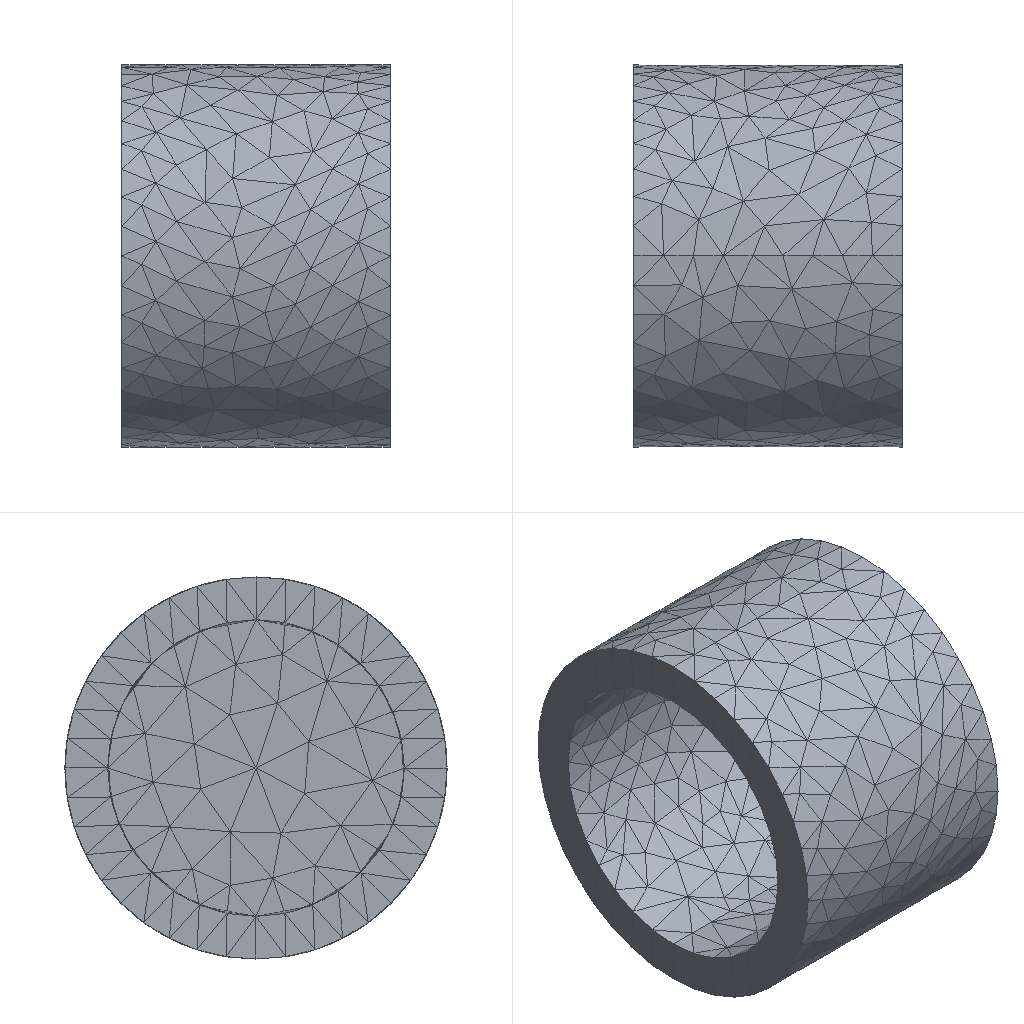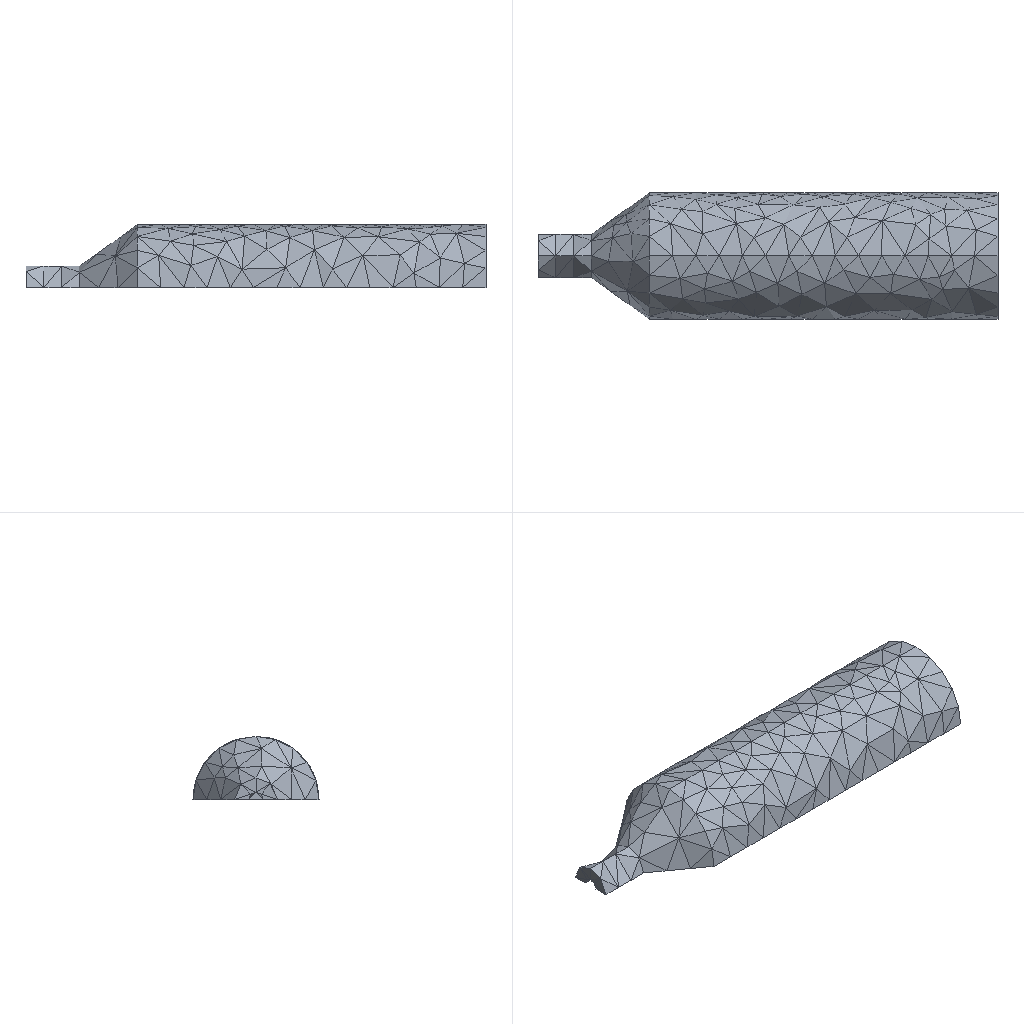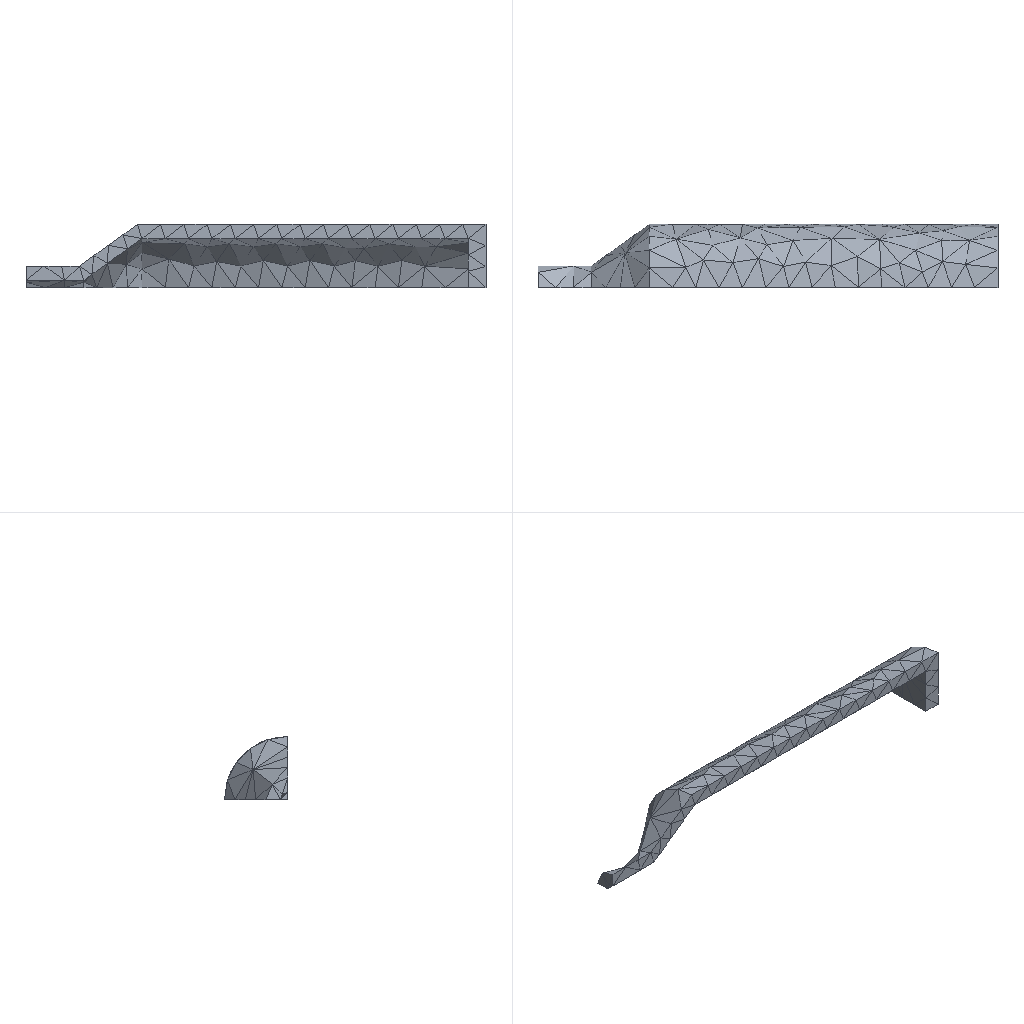Simulation study | ansys workbench
Set-up summary:
category,name,step,type,value,unit,region
solver,ansys_workbench
units,mm-N-s-tonne (MPa),,stated,"/units,MPA"
analysis,deck-1/LS1,,static
load_step,deck-1/LS1,deck-1/LS1,static,nsubst=1; time=1
analysis,deck-2/LS1,,static
load_step,deck-2/LS1,deck-2/LS1,static,nsubst=1; time=1
analysis,deck-3/LS1,,static
load_step,deck-3/LS1,deck-3/LS1,static,nsubst=1; time=1
mesh,deck-1.dat,,nodes,4195
mesh,deck-1.dat,,elements,3163
element_type,SOLID187,,,2247,,deck-1.dat
element_type,SURF154,,,916,,deck-1.dat
mesh,deck-2.dat,,nodes,1726
mesh,deck-2.dat,,elements,1182
element_type,SOLID187,,,784,,deck-2.dat
element_type,SURF154,,,398,,deck-2.dat
mesh,deck-3.dat,,nodes,887
mesh,deck-3.dat,,elements,550
element_type,SOLID187,,,368,,deck-3.dat
element_type,SURF154,,,182,,deck-3.dat
material,Structural Steel,,E,200000,tonne s^-2 mm^-1
material,Structural Steel,,nu,0.3
material,Structural Steel,,density,7.85e-09,tonne mm^-3
material,Structural Steel,,conductivity,60.5,tonne mm s^-3 C^-1
material,Structural Steel,,specific_heat,4.34e+08,mm^2 s^-2 C^-1
material,Structural Steel,,cte,1.2e-05,C^-1
material,Structural Steel,,permeability,10000
material,Structural Steel,,resistivity,0.00017,ohm mm
material,Structural Steel,,E,200000,tonne s^-2 mm^-1
material,Structural Steel,,nu,0.3
material,Structural Steel,,density,7.85e-09,tonne mm^-3
material,Structural Steel,,conductivity,60.5,tonne mm s^-3 C^-1
material,Structural Steel,,specific_heat,4.34e+08,mm^2 s^-2 C^-1
material,Structural Steel,,cte,1.2e-05,C^-1
material,Structural Steel,,permeability,10000
material,Structural Steel,,resistivity,0.00017,ohm mm
material,Structural Steel,,E,200000,tonne s^-2 mm^-1
material,Structural Steel,,nu,0.3
material,Structural Steel,,density,7.85e-09,tonne mm^-3
material,Structural Steel,,conductivity,60.5,tonne mm s^-3 C^-1
material,Structural Steel,,specific_heat,4.34e+08,mm^2 s^-2 C^-1
material,Structural Steel,,cte,1.2e-05,C^-1
material,Structural Steel,,permeability,10000
material,Structural Steel,,resistivity,0.00017,ohm mm
load,"Define Pressure Using Surface Effect Elements ""__""",deck-1/LS1,pressure,20,,SURF154 #2
load,"Define Pressure Using Surface Effect Elements ""__ 2""",deck-1/LS1,pressure,60,,SURF154 #3
load,"Define Pressure Using Surface Effect Elements ""__""",deck-2/LS1,pressure,20,,SURF154 #2
load,"Define Pressure Using Surface Effect Elements ""__ 2""",deck-2/LS1,pressure,60,,SURF154 #3
load,"Define Pressure Using Surface Effect Elements ""__""",deck-3/LS1,pressure,20,,SURF154 #2
load,"Define Pressure Using Surface Effect Elements ""__ 2""",deck-3/LS1,pressure,60,,SURF154 #3
bc,Fixed Supports,deck-1/model,fixed,[dofs=ALL],,_FIXEDSU
bc,Fixed Supports,deck-2/model,fixed,[dofs=ALL],,_FIXEDSU
bc,Fixed Supports,deck-3/model,fixed,[dofs=ALL],,_FIXEDSU
named_set,_FIXEDSU,,node,237
named_set,_FIXEDSU,,node,49
named_set,_FIXEDSU,,node,34
Results summary:
result,analyses[0].index,,,1
result,analyses[0].system,,,SYS
result,analyses[0].deck,,,deck-1.dat
result,analyses[0].solve_status,,,completed
result,analyses[0].analysis_type,,,static
result,analyses[0].physics,,,mechanical
result,analyses[0].unit_system,,,"NMM: mm, ton, N, s, mV, mA, degC"
result,analyses[0].n_sets,,,1
result,analyses[0].load_steps[0].set,set=1,,1
result,analyses[0].load_steps[0].time_or_freq,set=1,,1
result,analyses[0].load_steps[0].max_displacement_magnitude,set=1,,0.1222
result,analyses[0].load_steps[0].max_von_mises_nodal,set=1,,190.991
result,analyses[0].load_steps[0].reaction_force_sum_xyz[1],set=1,,8.91032e-09
result,analyses[0].load_steps[0].reaction_force_sum_xyz[2],set=1,,4.93112e-08
result,analyses[0].load_steps[0].reaction_force_sum_xyz[3],set=1,,2.93894e-08
result,analyses[1].index,,,2
result,analyses[1].system,,,SYS-1
result,analyses[1].deck,,,deck-2.dat
result,analyses[1].solve_status,,,completed
result,analyses[1].analysis_type,,,static
result,analyses[1].physics,,,mechanical
result,analyses[1].unit_system,,,"NMM: mm, ton, N, s, mV, mA, degC"
result,analyses[1].n_sets,,,1
result,analyses[1].load_steps[0].set,set=1,,1
result,analyses[1].load_steps[0].time_or_freq,set=1,,1
result,analyses[1].load_steps[0].max_displacement_magnitude,set=1,,149.547
result,analyses[1].load_steps[0].max_von_mises_nodal,set=1,,8405.59
result,analyses[1].load_steps[0].reaction_force_sum_xyz[1],set=1,,-6.56978e-06
result,analyses[1].load_steps[0].reaction_force_sum_xyz[2],set=1,,1.94181e-05
result,analyses[1].load_steps[0].reaction_force_sum_xyz[3],set=1,,-8.36629e+06
result,analyses[2].index,,,3
result,analyses[2].system,,,SYS-2
result,analyses[2].deck,,,deck-3.dat
result,analyses[2].solve_status,,,completed
result,analyses[2].analysis_type,,,static
result,analyses[2].physics,,,mechanical
result,analyses[2].unit_system,,,"NMM: mm, ton, N, s, mV, mA, degC"
result,analyses[2].n_sets,,,1
result,analyses[2].load_steps[0].set,set=1,,1
result,analyses[2].load_steps[0].time_or_freq,set=1,,1
result,analyses[2].load_steps[0].max_displacement_magnitude,set=1,,1602.23
result,analyses[2].load_steps[0].max_von_mises_nodal,set=1,,36587.5
result,analyses[2].load_steps[0].reaction_force_sum_xyz[1],set=1,,-0.0007552
result,analyses[2].load_steps[0].reaction_force_sum_xyz[2],set=1,,-4.18314e+06
result,analyses[2].load_steps[0].reaction_force_sum_xyz[3],set=1,,-4.18314e+06